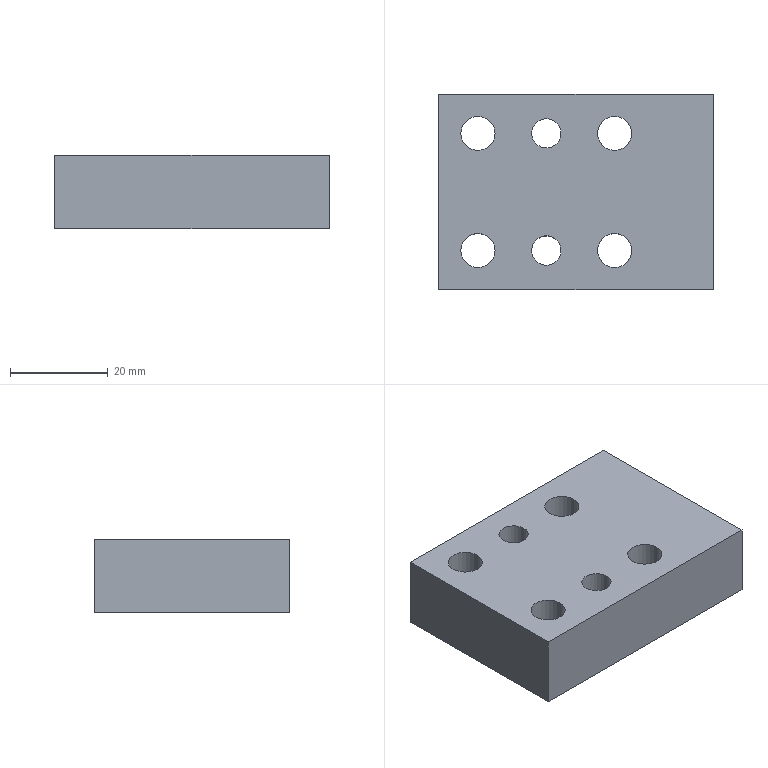Part | STEP file | Positioning_id1418_x_t | 1 solid | 18 faces | box 56.173 x 40 x 15 mm | volume 30547 mm3 | cylinder 12 | plane 6 | commonest cylinder face diameters 7 x8 6 x4